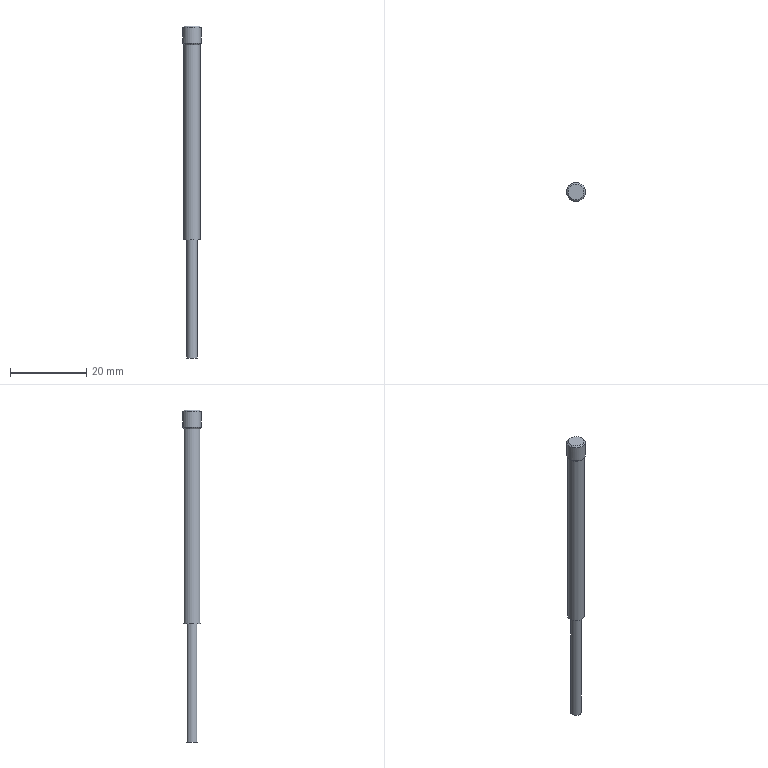Part | NX | features MI_APJAL_0254 2 | 1 solid | 9 faces | box 4.9 x 4.9 x 87 mm | volume 1059 mm3 | cylinder 3 | plane 3 | spline 2 | cone 1 | commonest cylinder face diameters 2.8 x1 4.4 x1 4.9 x1
STEP:
#1=CARTESIAN_POINT('',(1342.953,-79.442,73.1));
#2=VERTEX_POINT('',#1);
#3=CARTESIAN_POINT('',(1347.353,-79.442,73.1));
#4=VERTEX_POINT('',#3);
#5=CARTESIAN_POINT('',(1345.153,-79.442,73.1));
#6=DIRECTION('',(0.,0.,1.));
#7=DIRECTION('',(1.,0.,0.));
#8=AXIS2_PLACEMENT_3D('',#5,#6,#7);
#9=CIRCLE('',#8,2.2);
#10=EDGE_CURVE('',#2,#4,#9,.T.);
#11=ORIENTED_EDGE('',*,*,#10,.T.);
#12=CARTESIAN_POINT('',(1347.353,-79.44,73.1));
#13=VERTEX_POINT('',#12);
#14=CARTESIAN_POINT('',(1345.153,-79.442,73.1));
#15=DIRECTION('',(0.,0.,1.));
#16=DIRECTION('',(1.,0.,0.));
#17=AXIS2_PLACEMENT_3D('',#14,#15,#16);
#18=CIRCLE('',#17,2.2);
#19=EDGE_CURVE('',#4,#13,#18,.T.);
#20=ORIENTED_EDGE('',*,*,#19,.T.);
#21=CARTESIAN_POINT('',(1347.603,-79.44,73.448));
#22=VERTEX_POINT('',#21);
#23=CARTESIAN_POINT('',(1347.603,-79.44,73.448));
#24=DIRECTION('',(-0.5832,-0.0004724,-0.8123));
#25=VECTOR('',#24,1000.);
#26=LINE('',#23,#25);
#27=EDGE_CURVE('',#22,#13,#26,.T.);
#28=ORIENTED_EDGE('',*,*,#27,.F.);
#29=CARTESIAN_POINT('',(1347.603,-79.442,73.448));
#30=VERTEX_POINT('',#29);
#31=CARTESIAN_POINT('',(1347.603,-79.44,73.448));
#32=CARTESIAN_POINT('',(1347.603,-79.441,73.448));
#33=CARTESIAN_POINT('',(1347.603,-79.442,73.448));
#34=CARTESIAN_POINT('',(1347.603,-79.442,73.448));
#35=B_SPLINE_CURVE_WITH_KNOTS('',3,(#31,#32,#33,#34),.UNSPECIFIED.,.F.,.F.,(4,4),(13.004,13.006),.UNSPECIFIED.);
#36=EDGE_CURVE('',#22,#30,#35,.T.);
#37=ORIENTED_EDGE('',*,*,#36,.T.);
#38=CARTESIAN_POINT('',(1345.132,-81.892,73.448));
#39=VERTEX_POINT('',#38);
#40=CARTESIAN_POINT('',(1347.603,-79.442,73.448));
#41=CARTESIAN_POINT('',(1347.603,-79.758,73.448));
#42=CARTESIAN_POINT('',(1347.54,-80.08,73.448));
#43=CARTESIAN_POINT('',(1347.3,-80.665,73.448));
#44=CARTESIAN_POINT('',(1347.119,-80.938,73.448));
#45=CARTESIAN_POINT('',(1346.675,-81.388,73.448));
#46=CARTESIAN_POINT('',(1346.404,-81.573,73.448));
#47=CARTESIAN_POINT('',(1345.822,-81.82,73.448));
#48=CARTESIAN_POINT('',(1345.501,-81.888,73.448));
#49=CARTESIAN_POINT('',(1345.168,-81.892,73.448));
#50=CARTESIAN_POINT('',(1345.15,-81.892,73.448));
#51=CARTESIAN_POINT('',(1345.132,-81.892,73.448));
#52=B_SPLINE_CURVE_WITH_KNOTS('',3,(#40,#41,#42,#43,#44,#45,#46,#47,#48,#49,#50,#51),.UNSPECIFIED.,.F.,.F.,(4,2,2,2,2,4),(0.,0.8058,1.612,2.418,3.223,3.269),.UNSPECIFIED.);
#53=EDGE_CURVE('',#30,#39,#52,.T.);
#54=ORIENTED_EDGE('',*,*,#53,.T.);
#55=CARTESIAN_POINT('',(1342.703,-79.442,73.448));
#56=VERTEX_POINT('',#55);
#57=CARTESIAN_POINT('',(1345.132,-81.892,73.448));
#58=CARTESIAN_POINT('',(1344.833,-81.889,73.448));
#59=CARTESIAN_POINT('',(1344.53,-81.83,73.448));
#60=CARTESIAN_POINT('',(1343.959,-81.605,73.448));
#61=CARTESIAN_POINT('',(1343.683,-81.427,73.448));
#62=CARTESIAN_POINT('',(1343.227,-80.989,73.448));
#63=CARTESIAN_POINT('',(1343.039,-80.721,73.448));
#64=CARTESIAN_POINT('',(1342.784,-80.142,73.448));
#65=CARTESIAN_POINT('',(1342.712,-79.822,73.448));
#66=CARTESIAN_POINT('',(1342.704,-79.485,73.448));
#67=CARTESIAN_POINT('',(1342.703,-79.464,73.448));
#68=CARTESIAN_POINT('',(1342.703,-79.442,73.448));
#69=B_SPLINE_CURVE_WITH_KNOTS('',3,(#57,#58,#59,#60,#61,#62,#63,#64,#65,#66,#67,#68),.UNSPECIFIED.,.F.,.F.,(4,2,2,2,2,4),(3.269,4.029,4.835,5.641,6.447,6.501),.UNSPECIFIED.);
#70=EDGE_CURVE('',#39,#56,#69,.T.);
#71=ORIENTED_EDGE('',*,*,#70,.T.);
#72=CARTESIAN_POINT('',(1342.954,-79.442,73.1));
#73=CARTESIAN_POINT('',(1342.87,-79.442,73.216));
#74=CARTESIAN_POINT('',(1342.787,-79.442,73.332));
#75=CARTESIAN_POINT('',(1342.704,-79.442,73.449));
#76=B_SPLINE_CURVE_WITH_KNOTS('',3,(#72,#73,#74,#75),.UNSPECIFIED.,.F.,.F.,(4,4),(0.,1.),.UNSPECIFIED.);
#77=EDGE_CURVE('',#2,#56,#76,.T.);
#78=ORIENTED_EDGE('',*,*,#77,.F.);
#79=EDGE_LOOP('',(#11,#20,#28,#37,#54,#71,#78));
#80=FACE_BOUND('',#79,.T.);
#81=CARTESIAN_POINT('',(1342.954,-79.442,73.1));
#82=CARTESIAN_POINT('',(1342.87,-79.442,73.216));
#83=CARTESIAN_POINT('',(1342.787,-79.442,73.332));
#84=CARTESIAN_POINT('',(1342.704,-79.442,73.449));
#85=CARTESIAN_POINT('',(1342.954,-79.604,73.1));
#86=CARTESIAN_POINT('',(1342.87,-79.61,73.216));
#87=CARTESIAN_POINT('',(1342.787,-79.616,73.332));
#88=CARTESIAN_POINT('',(1342.704,-79.622,73.449));
#89=CARTESIAN_POINT('',(1342.972,-79.767,73.1));
#90=CARTESIAN_POINT('',(1342.889,-79.779,73.216));
#91=CARTESIAN_POINT('',(1342.806,-79.791,73.332));
#92=CARTESIAN_POINT('',(1342.724,-79.804,73.449));
#93=CARTESIAN_POINT('',(1343.043,-80.082,73.1));
#94=CARTESIAN_POINT('',(1342.963,-80.106,73.216));
#95=CARTESIAN_POINT('',(1342.883,-80.131,73.332));
#96=CARTESIAN_POINT('',(1342.803,-80.155,73.449));
#97=CARTESIAN_POINT('',(1343.096,-80.237,73.1));
#98=CARTESIAN_POINT('',(1343.018,-80.267,73.216));
#99=CARTESIAN_POINT('',(1342.94,-80.297,73.332));
#100=CARTESIAN_POINT('',(1342.862,-80.327,73.449));
#101=CARTESIAN_POINT('',(1343.286,-80.64,73.1));
#102=CARTESIAN_POINT('',(1343.216,-80.685,73.216));
#103=CARTESIAN_POINT('',(1343.145,-80.73,73.332));
#104=CARTESIAN_POINT('',(1343.074,-80.776,73.449));
#105=CARTESIAN_POINT('',(1343.462,-80.876,73.1));
#106=CARTESIAN_POINT('',(1343.397,-80.931,73.216));
#107=CARTESIAN_POINT('',(1343.333,-80.985,73.332));
#108=CARTESIAN_POINT('',(1343.269,-81.039,73.449));
#109=CARTESIAN_POINT('',(1343.881,-81.259,73.1));
#110=CARTESIAN_POINT('',(1343.833,-81.328,73.216));
#111=CARTESIAN_POINT('',(1343.784,-81.396,73.332));
#112=CARTESIAN_POINT('',(1343.736,-81.465,73.448));
#113=CARTESIAN_POINT('',(1344.133,-81.411,73.1));
#114=CARTESIAN_POINT('',(1344.094,-81.486,73.216));
#115=CARTESIAN_POINT('',(1344.055,-81.561,73.332));
#116=CARTESIAN_POINT('',(1344.017,-81.635,73.448));
#117=CARTESIAN_POINT('',(1344.666,-81.606,73.1));
#118=CARTESIAN_POINT('',(1344.647,-81.688,73.216));
#119=CARTESIAN_POINT('',(1344.629,-81.77,73.332));
#120=CARTESIAN_POINT('',(1344.611,-81.852,73.448));
#121=CARTESIAN_POINT('',(1344.957,-81.652,73.1));
#122=CARTESIAN_POINT('',(1344.949,-81.735,73.216));
#123=CARTESIAN_POINT('',(1344.942,-81.819,73.332));
#124=CARTESIAN_POINT('',(1344.935,-81.903,73.448));
#125=CARTESIAN_POINT('',(1345.524,-81.629,73.1));
#126=CARTESIAN_POINT('',(1345.538,-81.712,73.216));
#127=CARTESIAN_POINT('',(1345.552,-81.795,73.332));
#128=CARTESIAN_POINT('',(1345.566,-81.878,73.448));
#129=CARTESIAN_POINT('',(1345.81,-81.561,73.1));
#130=CARTESIAN_POINT('',(1345.835,-81.641,73.216));
#131=CARTESIAN_POINT('',(1345.86,-81.721,73.332));
#132=CARTESIAN_POINT('',(1345.885,-81.802,73.448));
#133=CARTESIAN_POINT('',(1346.327,-81.325,73.1));
#134=CARTESIAN_POINT('',(1346.371,-81.396,73.216));
#135=CARTESIAN_POINT('',(1346.415,-81.467,73.332));
#136=CARTESIAN_POINT('',(1346.46,-81.539,73.448));
#137=CARTESIAN_POINT('',(1346.566,-81.153,73.1));
#138=CARTESIAN_POINT('',(1346.619,-81.218,73.216));
#139=CARTESIAN_POINT('',(1346.673,-81.282,73.332));
#140=CARTESIAN_POINT('',(1346.726,-81.347,73.448));
#141=CARTESIAN_POINT('',(1346.954,-80.739,73.1));
#142=CARTESIAN_POINT('',(1347.022,-80.788,73.216));
#143=CARTESIAN_POINT('',(1347.09,-80.837,73.332));
#144=CARTESIAN_POINT('',(1347.158,-80.886,73.448));
#145=CARTESIAN_POINT('',(1347.109,-80.489,73.1));
#146=CARTESIAN_POINT('',(1347.184,-80.528,73.216));
#147=CARTESIAN_POINT('',(1347.258,-80.568,73.332));
#148=CARTESIAN_POINT('',(1347.332,-80.608,73.448));
#149=CARTESIAN_POINT('',(1347.311,-79.958,73.1));
#150=CARTESIAN_POINT('',(1347.393,-79.978,73.216));
#151=CARTESIAN_POINT('',(1347.474,-79.997,73.332));
#152=CARTESIAN_POINT('',(1347.556,-80.017,73.448));
#153=CARTESIAN_POINT('',(1347.36,-79.668,73.1));
#154=CARTESIAN_POINT('',(1347.444,-79.676,73.216));
#155=CARTESIAN_POINT('',(1347.528,-79.685,73.332));
#156=CARTESIAN_POINT('',(1347.611,-79.693,73.448));
#157=CARTESIAN_POINT('',(1347.345,-79.1,73.1));
#158=CARTESIAN_POINT('',(1347.428,-79.087,73.216));
#159=CARTESIAN_POINT('',(1347.511,-79.075,73.332));
#160=CARTESIAN_POINT('',(1347.594,-79.062,73.448));
#161=CARTESIAN_POINT('',(1347.281,-78.813,73.1));
#162=CARTESIAN_POINT('',(1347.361,-78.789,73.216));
#163=CARTESIAN_POINT('',(1347.442,-78.765,73.332));
#164=CARTESIAN_POINT('',(1347.523,-78.742,73.448));
#165=CARTESIAN_POINT('',(1347.052,-78.294,73.1));
#166=CARTESIAN_POINT('',(1347.123,-78.25,73.216));
#167=CARTESIAN_POINT('',(1347.195,-78.207,73.332));
#168=CARTESIAN_POINT('',(1347.267,-78.163,73.448));
#169=CARTESIAN_POINT('',(1346.883,-78.053,73.1));
#170=CARTESIAN_POINT('',(1346.948,-78.,73.216));
#171=CARTESIAN_POINT('',(1347.014,-77.947,73.332));
#172=CARTESIAN_POINT('',(1347.079,-77.895,73.448));
#173=CARTESIAN_POINT('',(1346.474,-77.659,73.1));
#174=CARTESIAN_POINT('',(1346.524,-77.592,73.216));
#175=CARTESIAN_POINT('',(1346.574,-77.524,73.332));
#176=CARTESIAN_POINT('',(1346.624,-77.457,73.448));
#177=CARTESIAN_POINT('',(1346.226,-77.5,73.1));
#178=CARTESIAN_POINT('',(1346.266,-77.427,73.216));
#179=CARTESIAN_POINT('',(1346.307,-77.353,73.332));
#180=CARTESIAN_POINT('',(1346.348,-77.279,73.448));
#181=CARTESIAN_POINT('',(1345.698,-77.292,73.1));
#182=CARTESIAN_POINT('',(1345.719,-77.21,73.216));
#183=CARTESIAN_POINT('',(1345.739,-77.129,73.332));
#184=CARTESIAN_POINT('',(1345.76,-77.047,73.448));
#185=CARTESIAN_POINT('',(1345.408,-77.239,73.1));
#186=CARTESIAN_POINT('',(1345.418,-77.155,73.216));
#187=CARTESIAN_POINT('',(1345.428,-77.072,73.332));
#188=CARTESIAN_POINT('',(1345.437,-76.988,73.448));
#189=CARTESIAN_POINT('',(1344.841,-77.246,73.1));
#190=CARTESIAN_POINT('',(1344.829,-77.163,73.216));
#191=CARTESIAN_POINT('',(1344.817,-77.08,73.332));
#192=CARTESIAN_POINT('',(1344.805,-76.996,73.448));
#193=CARTESIAN_POINT('',(1344.553,-77.307,73.1));
#194=CARTESIAN_POINT('',(1344.53,-77.226,73.216));
#195=CARTESIAN_POINT('',(1344.507,-77.145,73.332));
#196=CARTESIAN_POINT('',(1344.484,-77.064,73.448));
#197=CARTESIAN_POINT('',(1344.03,-77.529,73.1));
#198=CARTESIAN_POINT('',(1343.988,-77.457,73.216));
#199=CARTESIAN_POINT('',(1343.945,-77.384,73.332));
#200=CARTESIAN_POINT('',(1343.903,-77.312,73.448));
#201=CARTESIAN_POINT('',(1343.787,-77.695,73.1));
#202=CARTESIAN_POINT('',(1343.735,-77.629,73.216));
#203=CARTESIAN_POINT('',(1343.683,-77.562,73.332));
#204=CARTESIAN_POINT('',(1343.632,-77.496,73.448));
#205=CARTESIAN_POINT('',(1343.388,-78.099,73.1));
#206=CARTESIAN_POINT('',(1343.321,-78.048,73.216));
#207=CARTESIAN_POINT('',(1343.255,-77.997,73.332));
#208=CARTESIAN_POINT('',(1343.188,-77.946,73.448));
#209=CARTESIAN_POINT('',(1343.226,-78.344,73.1));
#210=CARTESIAN_POINT('',(1343.153,-78.303,73.216));
#211=CARTESIAN_POINT('',(1343.08,-78.261,73.332));
#212=CARTESIAN_POINT('',(1343.007,-78.22,73.448));
#213=CARTESIAN_POINT('',(1343.011,-78.87,73.1));
#214=CARTESIAN_POINT('',(1342.929,-78.848,73.216));
#215=CARTESIAN_POINT('',(1342.848,-78.826,73.332));
#216=CARTESIAN_POINT('',(1342.767,-78.804,73.448));
#217=CARTESIAN_POINT('',(1342.954,-79.158,73.1));
#218=CARTESIAN_POINT('',(1342.87,-79.148,73.216));
#219=CARTESIAN_POINT('',(1342.787,-79.137,73.332));
#220=CARTESIAN_POINT('',(1342.704,-79.126,73.448));
#221=CARTESIAN_POINT('',(1342.954,-79.442,73.1));
#222=CARTESIAN_POINT('',(1342.87,-79.442,73.216));
#223=CARTESIAN_POINT('',(1342.787,-79.442,73.332));
#224=CARTESIAN_POINT('',(1342.704,-79.442,73.449));
#225=B_SPLINE_SURFACE_WITH_KNOTS('',3,3,((#81,#82,#83,#84),(#85,#86,#87,#88),(#89,#90,#91,#92),(#93,#94,#95,#96),(#97,#98,#99,#100),(#101,#102,#103,#104),(#105,#106,#107,#108),(#109,#110,#111,#112),(#113,#114,#115,#116),(#117,#118,#119,#120),(#121,#122,#123,#124),(#125,#126,#127,#128),(#129,#130,#131,#132),(#133,#134,#135,#136),(#137,#138,#139,#140),(#141,#142,#143,#144),(#145,#146,#147,#148),(#149,#150,#151,#152),(#153,#154,#155,#156),(#157,#158,#159,#160),(#161,#162,#163,#164),(#165,#166,#167,#168),(#169,#170,#171,#172),(#173,#174,#175,#176),(#177,#178,#179,#180),(#181,#182,#183,#184),(#185,#186,#187,#188),(#189,#190,#191,#192),(#193,#194,#195,#196),(#197,#198,#199,#200),(#201,#202,#203,#204),(#205,#206,#207,#208),(#209,#210,#211,#212),(#213,#214,#215,#216),(#217,#218,#219,#220),(#221,#222,#223,#224)),.RULED_SURF.,.T.,.F.,.F.,(4,2,2,2,2,2,2,2,2,2,2,2,2,2,2,2,2,4),(4,4),(-13.006,-12.547,-12.088,-11.282,-10.476,-9.67,-8.864,-8.058,-7.253,-6.447,-5.641,-4.835,-4.029,-3.223,-2.418,-1.612,-0.8058,0.),(0.,1.),.UNSPECIFIED.);
#226=ADVANCED_FACE('',(#80),#225,.T.);
#227=CARTESIAN_POINT('',(1347.603,-79.456,77.633));
#228=VERTEX_POINT('',#227);
#229=CARTESIAN_POINT('',(1342.703,-79.442,77.633));
#230=VERTEX_POINT('',#229);
#231=CARTESIAN_POINT('',(1345.153,-79.442,77.633));
#232=DIRECTION('',(0.,0.,1.));
#233=DIRECTION('',(-1.,0.,0.));
#234=AXIS2_PLACEMENT_3D('',#231,#232,#233);
#235=CIRCLE('',#234,2.45);
#236=EDGE_CURVE('',#228,#230,#235,.T.);
#237=ORIENTED_EDGE('',*,*,#236,.F.);
#238=CARTESIAN_POINT('',(1345.132,-81.892,77.633));
#239=VERTEX_POINT('',#238);
#240=CARTESIAN_POINT('',(1345.153,-79.442,77.633));
#241=DIRECTION('',(0.,0.,1.));
#242=DIRECTION('',(-1.,0.,0.));
#243=AXIS2_PLACEMENT_3D('',#240,#241,#242);
#244=CIRCLE('',#243,2.45);
#245=EDGE_CURVE('',#239,#228,#244,.T.);
#246=ORIENTED_EDGE('',*,*,#245,.F.);
#247=CARTESIAN_POINT('',(1345.132,-81.892,77.632));
#248=CARTESIAN_POINT('',(1345.132,-81.892,73.448));
#249=B_SPLINE_CURVE_WITH_KNOTS('',1,(#247,#248),.UNSPECIFIED.,.F.,.F.,(2,2),(0.08333,0.9167),.UNSPECIFIED.);
#250=EDGE_CURVE('',#239,#39,#249,.T.);
#251=ORIENTED_EDGE('',*,*,#250,.T.);
#252=ORIENTED_EDGE('',*,*,#53,.F.);
#253=ORIENTED_EDGE('',*,*,#36,.F.);
#254=CARTESIAN_POINT('',(1342.703,-79.442,73.448));
#255=CARTESIAN_POINT('',(1342.704,-79.147,73.448));
#256=CARTESIAN_POINT('',(1342.758,-78.847,73.448));
#257=CARTESIAN_POINT('',(1342.975,-78.276,73.448));
#258=CARTESIAN_POINT('',(1343.149,-77.998,73.448));
#259=CARTESIAN_POINT('',(1343.581,-77.537,73.448));
#260=CARTESIAN_POINT('',(1343.847,-77.345,73.448));
#261=CARTESIAN_POINT('',(1344.422,-77.083,73.448));
#262=CARTESIAN_POINT('',(1344.741,-77.007,73.448));
#263=CARTESIAN_POINT('',(1345.373,-76.982,73.448));
#264=CARTESIAN_POINT('',(1345.697,-77.032,73.448));
#265=CARTESIAN_POINT('',(1346.29,-77.249,73.448));
#266=CARTESIAN_POINT('',(1346.571,-77.419,73.448));
#267=CARTESIAN_POINT('',(1347.038,-77.845,73.448));
#268=CARTESIAN_POINT('',(1347.233,-78.109,73.448));
#269=CARTESIAN_POINT('',(1347.445,-78.557,73.448));
#270=CARTESIAN_POINT('',(1347.504,-78.73,73.448));
#271=CARTESIAN_POINT('',(1347.583,-79.08,73.448));
#272=CARTESIAN_POINT('',(1347.603,-79.261,73.448));
#273=CARTESIAN_POINT('',(1347.603,-79.44,73.448));
#274=B_SPLINE_CURVE_WITH_KNOTS('',3,(#254,#255,#256,#257,#258,#259,#260,#261,#262,#263,#264,#265,#266,#267,#268,#269,#270,#271,#272,#273),.UNSPECIFIED.,.F.,.F.,(4,2,2,2,2,2,2,2,2,4),(6.501,7.253,8.058,8.864,9.67,10.476,11.282,12.088,12.547,13.004),.UNSPECIFIED.);
#275=EDGE_CURVE('',#56,#22,#274,.T.);
#276=ORIENTED_EDGE('',*,*,#275,.F.);
#277=ORIENTED_EDGE('',*,*,#70,.F.);
#278=ORIENTED_EDGE('',*,*,#250,.F.);
#279=CARTESIAN_POINT('',(1345.153,-79.442,77.633));
#280=DIRECTION('',(0.,0.,1.));
#281=DIRECTION('',(-1.,0.,0.));
#282=AXIS2_PLACEMENT_3D('',#279,#280,#281);
#283=CIRCLE('',#282,2.45);
#284=EDGE_CURVE('',#230,#239,#283,.T.);
#285=ORIENTED_EDGE('',*,*,#284,.F.);
#286=EDGE_LOOP('',(#237,#246,#251,#252,#253,#276,#277,#278,#285));
#287=FACE_BOUND('',#286,.T.);
#288=CARTESIAN_POINT('',(1345.153,-79.442,75.55));
#289=DIRECTION('',(0.,0.,-1.));
#290=DIRECTION('',(-0.008727,-1.,0.));
#291=AXIS2_PLACEMENT_3D('',#288,#289,#290);
#292=CYLINDRICAL_SURFACE('',#291,2.45);
#293=ADVANCED_FACE('',(#287),#292,.T.);
#294=CARTESIAN_POINT('',(1343.071,-79.442,78.));
#295=VERTEX_POINT('',#294);
#296=CARTESIAN_POINT('',(1347.236,-79.454,78.));
#297=VERTEX_POINT('',#296);
#298=CARTESIAN_POINT('',(1345.153,-79.442,78.));
#299=DIRECTION('',(0.,0.,-1.));
#300=DIRECTION('',(-1.,0.,0.));
#301=AXIS2_PLACEMENT_3D('',#298,#299,#300);
#302=CIRCLE('',#301,2.083);
#303=EDGE_CURVE('',#295,#297,#302,.T.);
#304=ORIENTED_EDGE('',*,*,#303,.T.);
#305=CARTESIAN_POINT('',(1347.236,-79.454,78.));
#306=CARTESIAN_POINT('',(1347.603,-79.456,77.633));
#307=B_SPLINE_CURVE_WITH_KNOTS('',1,(#305,#306),.UNSPECIFIED.,.F.,.F.,(2,2),(0.601,0.7071),.UNSPECIFIED.);
#308=EDGE_CURVE('',#297,#228,#307,.T.);
#309=ORIENTED_EDGE('',*,*,#308,.T.);
#310=ORIENTED_EDGE('',*,*,#236,.T.);
#311=ORIENTED_EDGE('',*,*,#284,.T.);
#312=ORIENTED_EDGE('',*,*,#245,.T.);
#313=ORIENTED_EDGE('',*,*,#308,.F.);
#314=CARTESIAN_POINT('',(1345.153,-79.442,78.));
#315=DIRECTION('',(0.,0.,-1.));
#316=DIRECTION('',(-1.,0.,0.));
#317=AXIS2_PLACEMENT_3D('',#314,#315,#316);
#318=CIRCLE('',#317,2.083);
#319=EDGE_CURVE('',#297,#295,#318,.T.);
#320=ORIENTED_EDGE('',*,*,#319,.T.);
#321=EDGE_LOOP('',(#304,#309,#310,#311,#312,#313,#320));
#322=FACE_BOUND('',#321,.T.);
#323=CARTESIAN_POINT('',(1345.153,-79.442,76.618));
#324=DIRECTION('',(0.,0.,-1.));
#325=DIRECTION('',(1.,-0.005818,0.));
#326=AXIS2_PLACEMENT_3D('',#323,#324,#325);
#327=CONICAL_SURFACE('',#326,3.465,0.7854);
#328=ADVANCED_FACE('',(#322),#327,.T.);
#329=ORIENTED_EDGE('',*,*,#319,.F.);
#330=ORIENTED_EDGE('',*,*,#303,.F.);
#331=EDGE_LOOP('',(#329,#330));
#332=FACE_BOUND('',#331,.T.);
#333=CARTESIAN_POINT('',(1342.446,-83.771,78.));
#334=DIRECTION('',(0.,0.,1.));
#335=DIRECTION('',(1.,0.,0.));
#336=AXIS2_PLACEMENT_3D('',#333,#334,#335);
#337=PLANE('',#336);
#338=ADVANCED_FACE('',(#332),#337,.T.);
#339=CARTESIAN_POINT('',(1343.753,-79.442,22.));
#340=VERTEX_POINT('',#339);
#341=CARTESIAN_POINT('',(1345.153,-79.442,22.));
#342=DIRECTION('',(0.,0.,1.));
#343=DIRECTION('',(-1.,0.,0.));
#344=AXIS2_PLACEMENT_3D('',#341,#342,#343);
#345=CIRCLE('',#344,1.4);
#346=EDGE_CURVE('',#340,#340,#345,.T.);
#347=ORIENTED_EDGE('',*,*,#346,.F.);
#348=CARTESIAN_POINT('',(1343.753,-79.442,-9.));
#349=VERTEX_POINT('',#348);
#350=CARTESIAN_POINT('',(1343.753,-79.442,22.));
#351=CARTESIAN_POINT('',(1343.753,-79.442,-9.));
#352=B_SPLINE_CURVE_WITH_KNOTS('',1,(#350,#351),.UNSPECIFIED.,.F.,.F.,(2,2),(0.08333,0.9167),.UNSPECIFIED.);
#353=EDGE_CURVE('',#340,#349,#352,.T.);
#354=ORIENTED_EDGE('',*,*,#353,.T.);
#355=CARTESIAN_POINT('',(1345.153,-79.442,-9.));
#356=DIRECTION('',(0.,0.,-1.));
#357=DIRECTION('',(-1.,0.,0.));
#358=AXIS2_PLACEMENT_3D('',#355,#356,#357);
#359=CIRCLE('',#358,1.4);
#360=EDGE_CURVE('',#349,#349,#359,.T.);
#361=ORIENTED_EDGE('',*,*,#360,.F.);
#362=ORIENTED_EDGE('',*,*,#353,.F.);
#363=EDGE_LOOP('',(#347,#354,#361,#362));
#364=FACE_BOUND('',#363,.T.);
#365=CARTESIAN_POINT('',(1345.153,-79.442,6.5));
#366=DIRECTION('',(0.,0.,-1.));
#367=DIRECTION('',(-1.,0.,0.));
#368=AXIS2_PLACEMENT_3D('',#365,#366,#367);
#369=CYLINDRICAL_SURFACE('',#368,1.4);
#370=ADVANCED_FACE('',(#364),#369,.T.);
#371=ORIENTED_EDGE('',*,*,#360,.T.);
#372=EDGE_LOOP('',(#371));
#373=FACE_BOUND('',#372,.T.);
#374=CARTESIAN_POINT('',(1348.373,-82.352,-9.));
#375=DIRECTION('',(0.,0.,-1.));
#376=DIRECTION('',(-1.,0.,0.));
#377=AXIS2_PLACEMENT_3D('',#374,#375,#376);
#378=PLANE('',#377);
#379=ADVANCED_FACE('',(#373),#378,.T.);
#380=ORIENTED_EDGE('',*,*,#10,.F.);
#381=CARTESIAN_POINT('',(1342.953,-79.442,22.));
#382=VERTEX_POINT('',#381);
#383=CARTESIAN_POINT('',(1342.953,-79.442,73.1));
#384=CARTESIAN_POINT('',(1342.953,-79.442,22.));
#385=B_SPLINE_CURVE_WITH_KNOTS('',1,(#383,#384),.UNSPECIFIED.,.F.,.F.,(2,2),(0.08333,0.9167),.UNSPECIFIED.);
#386=EDGE_CURVE('',#2,#382,#385,.T.);
#387=ORIENTED_EDGE('',*,*,#386,.T.);
#388=CARTESIAN_POINT('',(1345.153,-79.442,22.));
#389=DIRECTION('',(0.,0.,-1.));
#390=DIRECTION('',(-1.,0.,0.));
#391=AXIS2_PLACEMENT_3D('',#388,#389,#390);
#392=CIRCLE('',#391,2.2);
#393=EDGE_CURVE('',#382,#382,#392,.T.);
#394=ORIENTED_EDGE('',*,*,#393,.F.);
#395=ORIENTED_EDGE('',*,*,#386,.F.);
#396=CARTESIAN_POINT('',(1345.153,-79.442,73.1));
#397=DIRECTION('',(0.,0.,1.));
#398=DIRECTION('',(1.,0.,0.));
#399=AXIS2_PLACEMENT_3D('',#396,#397,#398);
#400=CIRCLE('',#399,2.2);
#401=EDGE_CURVE('',#13,#2,#400,.T.);
#402=ORIENTED_EDGE('',*,*,#401,.F.);
#403=ORIENTED_EDGE('',*,*,#19,.F.);
#404=EDGE_LOOP('',(#380,#387,#394,#395,#402,#403));
#405=FACE_BOUND('',#404,.T.);
#406=CARTESIAN_POINT('',(1345.153,-79.442,47.55));
#407=DIRECTION('',(0.,0.,-1.));
#408=DIRECTION('',(-1.,0.,0.));
#409=AXIS2_PLACEMENT_3D('',#406,#407,#408);
#410=CYLINDRICAL_SURFACE('',#409,2.2);
#411=ADVANCED_FACE('',(#405),#410,.T.);
#412=ORIENTED_EDGE('',*,*,#393,.T.);
#413=EDGE_LOOP('',(#412));
#414=FACE_BOUND('',#413,.T.);
#415=ORIENTED_EDGE('',*,*,#346,.T.);
#416=EDGE_LOOP('',(#415));
#417=FACE_BOUND('',#416,.T.);
#418=CARTESIAN_POINT('',(1350.213,-84.015,22.));
#419=DIRECTION('',(0.,0.,-1.));
#420=DIRECTION('',(-1.,0.,0.));
#421=AXIS2_PLACEMENT_3D('',#418,#419,#420);
#422=PLANE('',#421);
#423=ADVANCED_FACE('',(#414,#417),#422,.T.);
#424=ORIENTED_EDGE('',*,*,#275,.T.);
#425=ORIENTED_EDGE('',*,*,#27,.T.);
#426=ORIENTED_EDGE('',*,*,#401,.T.);
#427=ORIENTED_EDGE('',*,*,#77,.T.);
#428=EDGE_LOOP('',(#424,#425,#426,#427));
#429=FACE_BOUND('',#428,.T.);
#430=CARTESIAN_POINT('',(1342.954,-79.442,73.1));
#431=CARTESIAN_POINT('',(1342.87,-79.442,73.216));
#432=CARTESIAN_POINT('',(1342.787,-79.442,73.332));
#433=CARTESIAN_POINT('',(1342.704,-79.442,73.449));
#434=CARTESIAN_POINT('',(1342.954,-79.604,73.1));
#435=CARTESIAN_POINT('',(1342.87,-79.61,73.216));
#436=CARTESIAN_POINT('',(1342.787,-79.616,73.332));
#437=CARTESIAN_POINT('',(1342.704,-79.622,73.449));
#438=CARTESIAN_POINT('',(1342.972,-79.767,73.1));
#439=CARTESIAN_POINT('',(1342.889,-79.779,73.216));
#440=CARTESIAN_POINT('',(1342.806,-79.791,73.332));
#441=CARTESIAN_POINT('',(1342.724,-79.804,73.449));
#442=CARTESIAN_POINT('',(1343.043,-80.082,73.1));
#443=CARTESIAN_POINT('',(1342.963,-80.106,73.216));
#444=CARTESIAN_POINT('',(1342.883,-80.131,73.332));
#445=CARTESIAN_POINT('',(1342.803,-80.155,73.449));
#446=CARTESIAN_POINT('',(1343.096,-80.237,73.1));
#447=CARTESIAN_POINT('',(1343.018,-80.267,73.216));
#448=CARTESIAN_POINT('',(1342.94,-80.297,73.332));
#449=CARTESIAN_POINT('',(1342.862,-80.327,73.449));
#450=CARTESIAN_POINT('',(1343.286,-80.64,73.1));
#451=CARTESIAN_POINT('',(1343.216,-80.685,73.216));
#452=CARTESIAN_POINT('',(1343.145,-80.73,73.332));
#453=CARTESIAN_POINT('',(1343.074,-80.776,73.449));
#454=CARTESIAN_POINT('',(1343.462,-80.876,73.1));
#455=CARTESIAN_POINT('',(1343.397,-80.931,73.216));
#456=CARTESIAN_POINT('',(1343.333,-80.985,73.332));
#457=CARTESIAN_POINT('',(1343.269,-81.039,73.449));
#458=CARTESIAN_POINT('',(1343.881,-81.259,73.1));
#459=CARTESIAN_POINT('',(1343.833,-81.328,73.216));
#460=CARTESIAN_POINT('',(1343.784,-81.396,73.332));
#461=CARTESIAN_POINT('',(1343.736,-81.465,73.448));
#462=CARTESIAN_POINT('',(1344.133,-81.411,73.1));
#463=CARTESIAN_POINT('',(1344.094,-81.486,73.216));
#464=CARTESIAN_POINT('',(1344.055,-81.561,73.332));
#465=CARTESIAN_POINT('',(1344.017,-81.635,73.448));
#466=CARTESIAN_POINT('',(1344.666,-81.606,73.1));
#467=CARTESIAN_POINT('',(1344.647,-81.688,73.216));
#468=CARTESIAN_POINT('',(1344.629,-81.77,73.332));
#469=CARTESIAN_POINT('',(1344.611,-81.852,73.448));
#470=CARTESIAN_POINT('',(1344.957,-81.652,73.1));
#471=CARTESIAN_POINT('',(1344.949,-81.735,73.216));
#472=CARTESIAN_POINT('',(1344.942,-81.819,73.332));
#473=CARTESIAN_POINT('',(1344.935,-81.903,73.448));
#474=CARTESIAN_POINT('',(1345.524,-81.629,73.1));
#475=CARTESIAN_POINT('',(1345.538,-81.712,73.216));
#476=CARTESIAN_POINT('',(1345.552,-81.795,73.332));
#477=CARTESIAN_POINT('',(1345.566,-81.878,73.448));
#478=CARTESIAN_POINT('',(1345.81,-81.561,73.1));
#479=CARTESIAN_POINT('',(1345.835,-81.641,73.216));
#480=CARTESIAN_POINT('',(1345.86,-81.721,73.332));
#481=CARTESIAN_POINT('',(1345.885,-81.802,73.448));
#482=CARTESIAN_POINT('',(1346.327,-81.325,73.1));
#483=CARTESIAN_POINT('',(1346.371,-81.396,73.216));
#484=CARTESIAN_POINT('',(1346.415,-81.467,73.332));
#485=CARTESIAN_POINT('',(1346.46,-81.539,73.448));
#486=CARTESIAN_POINT('',(1346.566,-81.153,73.1));
#487=CARTESIAN_POINT('',(1346.619,-81.218,73.216));
#488=CARTESIAN_POINT('',(1346.673,-81.282,73.332));
#489=CARTESIAN_POINT('',(1346.726,-81.347,73.448));
#490=CARTESIAN_POINT('',(1346.954,-80.739,73.1));
#491=CARTESIAN_POINT('',(1347.022,-80.788,73.216));
#492=CARTESIAN_POINT('',(1347.09,-80.837,73.332));
#493=CARTESIAN_POINT('',(1347.158,-80.886,73.448));
#494=CARTESIAN_POINT('',(1347.109,-80.489,73.1));
#495=CARTESIAN_POINT('',(1347.184,-80.528,73.216));
#496=CARTESIAN_POINT('',(1347.258,-80.568,73.332));
#497=CARTESIAN_POINT('',(1347.332,-80.608,73.448));
#498=CARTESIAN_POINT('',(1347.311,-79.958,73.1));
#499=CARTESIAN_POINT('',(1347.393,-79.978,73.216));
#500=CARTESIAN_POINT('',(1347.474,-79.997,73.332));
#501=CARTESIAN_POINT('',(1347.556,-80.017,73.448));
#502=CARTESIAN_POINT('',(1347.36,-79.668,73.1));
#503=CARTESIAN_POINT('',(1347.444,-79.676,73.216));
#504=CARTESIAN_POINT('',(1347.528,-79.685,73.332));
#505=CARTESIAN_POINT('',(1347.611,-79.693,73.448));
#506=CARTESIAN_POINT('',(1347.345,-79.1,73.1));
#507=CARTESIAN_POINT('',(1347.428,-79.087,73.216));
#508=CARTESIAN_POINT('',(1347.511,-79.075,73.332));
#509=CARTESIAN_POINT('',(1347.594,-79.062,73.448));
#510=CARTESIAN_POINT('',(1347.281,-78.813,73.1));
#511=CARTESIAN_POINT('',(1347.361,-78.789,73.216));
#512=CARTESIAN_POINT('',(1347.442,-78.765,73.332));
#513=CARTESIAN_POINT('',(1347.523,-78.742,73.448));
#514=CARTESIAN_POINT('',(1347.052,-78.294,73.1));
#515=CARTESIAN_POINT('',(1347.123,-78.25,73.216));
#516=CARTESIAN_POINT('',(1347.195,-78.207,73.332));
#517=CARTESIAN_POINT('',(1347.267,-78.163,73.448));
#518=CARTESIAN_POINT('',(1346.883,-78.053,73.1));
#519=CARTESIAN_POINT('',(1346.948,-78.,73.216));
#520=CARTESIAN_POINT('',(1347.014,-77.947,73.332));
#521=CARTESIAN_POINT('',(1347.079,-77.895,73.448));
#522=CARTESIAN_POINT('',(1346.474,-77.659,73.1));
#523=CARTESIAN_POINT('',(1346.524,-77.592,73.216));
#524=CARTESIAN_POINT('',(1346.574,-77.524,73.332));
#525=CARTESIAN_POINT('',(1346.624,-77.457,73.448));
#526=CARTESIAN_POINT('',(1346.226,-77.5,73.1));
#527=CARTESIAN_POINT('',(1346.266,-77.427,73.216));
#528=CARTESIAN_POINT('',(1346.307,-77.353,73.332));
#529=CARTESIAN_POINT('',(1346.348,-77.279,73.448));
#530=CARTESIAN_POINT('',(1345.698,-77.292,73.1));
#531=CARTESIAN_POINT('',(1345.719,-77.21,73.216));
#532=CARTESIAN_POINT('',(1345.739,-77.129,73.332));
#533=CARTESIAN_POINT('',(1345.76,-77.047,73.448));
#534=CARTESIAN_POINT('',(1345.408,-77.239,73.1));
#535=CARTESIAN_POINT('',(1345.418,-77.155,73.216));
#536=CARTESIAN_POINT('',(1345.428,-77.072,73.332));
#537=CARTESIAN_POINT('',(1345.437,-76.988,73.448));
#538=CARTESIAN_POINT('',(1344.841,-77.246,73.1));
#539=CARTESIAN_POINT('',(1344.829,-77.163,73.216));
#540=CARTESIAN_POINT('',(1344.817,-77.08,73.332));
#541=CARTESIAN_POINT('',(1344.805,-76.996,73.448));
#542=CARTESIAN_POINT('',(1344.553,-77.307,73.1));
#543=CARTESIAN_POINT('',(1344.53,-77.226,73.216));
#544=CARTESIAN_POINT('',(1344.507,-77.145,73.332));
#545=CARTESIAN_POINT('',(1344.484,-77.064,73.448));
#546=CARTESIAN_POINT('',(1344.03,-77.529,73.1));
#547=CARTESIAN_POINT('',(1343.988,-77.457,73.216));
#548=CARTESIAN_POINT('',(1343.945,-77.384,73.332));
#549=CARTESIAN_POINT('',(1343.903,-77.312,73.448));
#550=CARTESIAN_POINT('',(1343.787,-77.695,73.1));
#551=CARTESIAN_POINT('',(1343.735,-77.629,73.216));
#552=CARTESIAN_POINT('',(1343.683,-77.562,73.332));
#553=CARTESIAN_POINT('',(1343.632,-77.496,73.448));
#554=CARTESIAN_POINT('',(1343.388,-78.099,73.1));
#555=CARTESIAN_POINT('',(1343.321,-78.048,73.216));
#556=CARTESIAN_POINT('',(1343.255,-77.997,73.332));
#557=CARTESIAN_POINT('',(1343.188,-77.946,73.448));
#558=CARTESIAN_POINT('',(1343.226,-78.344,73.1));
#559=CARTESIAN_POINT('',(1343.153,-78.303,73.216));
#560=CARTESIAN_POINT('',(1343.08,-78.261,73.332));
#561=CARTESIAN_POINT('',(1343.007,-78.22,73.448));
#562=CARTESIAN_POINT('',(1343.011,-78.87,73.1));
#563=CARTESIAN_POINT('',(1342.929,-78.848,73.216));
#564=CARTESIAN_POINT('',(1342.848,-78.826,73.332));
#565=CARTESIAN_POINT('',(1342.767,-78.804,73.448));
#566=CARTESIAN_POINT('',(1342.954,-79.158,73.1));
#567=CARTESIAN_POINT('',(1342.87,-79.148,73.216));
#568=CARTESIAN_POINT('',(1342.787,-79.137,73.332));
#569=CARTESIAN_POINT('',(1342.704,-79.126,73.448));
#570=CARTESIAN_POINT('',(1342.954,-79.442,73.1));
#571=CARTESIAN_POINT('',(1342.87,-79.442,73.216));
#572=CARTESIAN_POINT('',(1342.787,-79.442,73.332));
#573=CARTESIAN_POINT('',(1342.704,-79.442,73.449));
#574=B_SPLINE_SURFACE_WITH_KNOTS('',3,3,((#430,#431,#432,#433),(#434,#435,#436,#437),(#438,#439,#440,#441),(#442,#443,#444,#445),(#446,#447,#448,#449),(#450,#451,#452,#453),(#454,#455,#456,#457),(#458,#459,#460,#461),(#462,#463,#464,#465),(#466,#467,#468,#469),(#470,#471,#472,#473),(#474,#475,#476,#477),(#478,#479,#480,#481),(#482,#483,#484,#485),(#486,#487,#488,#489),(#490,#491,#492,#493),(#494,#495,#496,#497),(#498,#499,#500,#501),(#502,#503,#504,#505),(#506,#507,#508,#509),(#510,#511,#512,#513),(#514,#515,#516,#517),(#518,#519,#520,#521),(#522,#523,#524,#525),(#526,#527,#528,#529),(#530,#531,#532,#533),(#534,#535,#536,#537),(#538,#539,#540,#541),(#542,#543,#544,#545),(#546,#547,#548,#549),(#550,#551,#552,#553),(#554,#555,#556,#557),(#558,#559,#560,#561),(#562,#563,#564,#565),(#566,#567,#568,#569),(#570,#571,#572,#573)),.RULED_SURF.,.T.,.F.,.F.,(4,2,2,2,2,2,2,2,2,2,2,2,2,2,2,2,2,4),(4,4),(-13.006,-12.547,-12.088,-11.282,-10.476,-9.67,-8.864,-8.058,-7.253,-6.447,-5.641,-4.835,-4.029,-3.223,-2.418,-1.612,-0.8058,0.),(0.,1.),.UNSPECIFIED.);
#575=ADVANCED_FACE('',(#429),#574,.T.);
#576=CLOSED_SHELL('',(#226,#293,#328,#338,#370,#379,#411,#423,#575));
#577=MANIFOLD_SOLID_BREP('',#576);
#578=(LENGTH_UNIT()NAMED_UNIT(*)SI_UNIT(.MILLI.,.METRE.));
#579=UNCERTAINTY_MEASURE_WITH_UNIT(LENGTH_MEASURE(0.00001),#578,'','');
#580=(NAMED_UNIT(*)PLANE_ANGLE_UNIT()SI_UNIT($,.RADIAN.));
#581=(NAMED_UNIT(*)SI_UNIT($,.STERADIAN.)SOLID_ANGLE_UNIT());
#582=(GEOMETRIC_REPRESENTATION_CONTEXT(3)GLOBAL_UNCERTAINTY_ASSIGNED_CONTEXT((#579))GLOBAL_UNIT_ASSIGNED_CONTEXT((#578,#580,#581))REPRESENTATION_CONTEXT('',''));
#583=ADVANCED_BREP_SHAPE_REPRESENTATION('',(#577),#582);